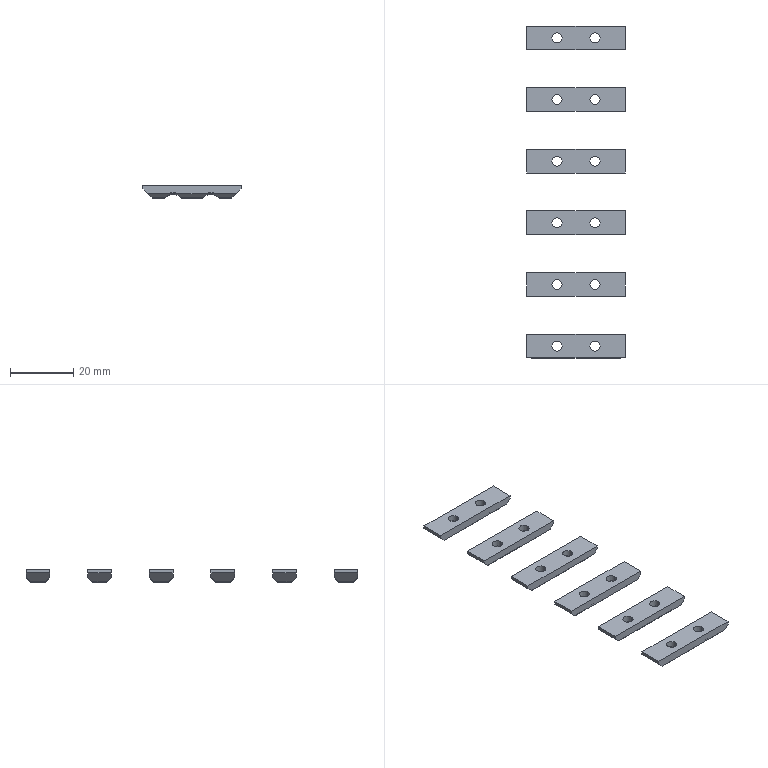NC program | NX | posted with a generic post | part box 31 x 105 x 4 mm
Lines 1 to 1424 of 12738:
N10 G17 G21 G94 G90
(FLOOR_WALL_COPY , TOOL : D10JING)
N12 T14 M6
N14 G54
N16 G17 G0 G90 X-65.5 Y18.497 S9500 M3
N18 G43 Z30. H14
N20 Z4.
N22 G94 G1 Z1. F1500.
N24 X-60.5
N26 X60.5
N28 Y11.898
N30 X-60.5
N32 Y5.298
N34 X60.5
N36 Y-1.301
N38 X-60.5
N40 Y-7.901
N42 X60.5
N44 Y-14.5
N46 X-60.5
N48 X-65.5
N50 Z4.
N52 G0 Z30.
N54 Y18.497
N56 Z3.
N58 G1 Z0.
N60 X-60.5
N62 X60.5
N64 Y11.898
N66 X-60.5
N68 Y5.298
N70 X60.5
N72 Y-1.301
N74 X-60.5
N76 Y-7.901
N78 X60.5
N80 Y-14.5
N82 X-60.5
N84 X-65.5
N86 Z3.
N88 G0 Z30.
N90 M5
(ZLEVEL_PROFILE_1 , TOOL : D10)
N92 T15 M6
N94 G54
N96 G17 G0 G90 X39.9 Y9.729 S9500 M3
N98 G43 Z30. H15
N100 Z1.5
N102 G94 G1 Y16.054 Z1.169 F1000.
N104 X40.234 Y17.398 Z1.096
N106 X40.916 Y18.604 Z1.023
N108 X41.896 Y19.584 Z0.951
N110 X43.102 Y20.266 Z0.878
N112 X44.446 Y20.6 Z0.805
N114 X53.054 Z0.354
N116 X54.398 Y20.266 Z0.282
N118 X55.604 Y19.584 Z0.209
N120 X56.584 Y18.604 Z0.137
N122 X57.266 Y17.398 Z0.064
N124 X57.6 Y16.054 Z-0.009
N126 Y0. Z-0.85
N128 Y-15.5 F2500.
N130 G2 X52.5 Y-20.6 R5.1
N132 G1 X45.
N134 G2 X39.9 Y-15.5 R5.1
N136 G1 Y15.5
N138 G2 X45. Y20.6 R5.1
N140 G1 X52.5
N142 G2 X57.6 Y15.5 R5.1
N144 G1 Y0.
N146 Y-15.459 Z-1.12
N148 X57.588 Y-15.845 Z-1.127
N150 X57.548 Y-16.23 Z-1.133
N152 X57.478 Y-16.61 Z-1.14
N154 X57.38 Y-16.983 Z-1.147
N156 X57.253 Y-17.349 Z-1.154
N158 X57.1 Y-17.703 Z-1.16
N160 X56.92 Y-18.045 Z-1.167
N162 X56.714 Y-18.372 Z-1.174
N164 X56.485 Y-18.683 Z-1.181
N166 X56.232 Y-18.976 Z-1.187
N168 X55.958 Y-19.248 Z-1.194
N170 X55.665 Y-19.499 Z-1.201
N172 X55.353 Y-19.727 Z-1.208
N174 X55.025 Y-19.931 Z-1.214
N176 X54.682 Y-20.11 Z-1.221
N178 X54.327 Y-20.262 Z-1.228
N180 X53.961 Y-20.386 Z-1.235
N182 X53.587 Y-20.483 Z-1.241
N184 X53.206 Y-20.551 Z-1.248
N186 X52.822 Y-20.59 Z-1.255
N188 X52.436 Y-20.6 Z-1.262
N190 X52.049 Z-1.268
N192 X45.093 Z-1.39
N194 X44.706 Y-20.592 Z-1.396
N196 X44.322 Y-20.555 Z-1.403
N198 X43.941 Y-20.489 Z-1.41
N200 X43.566 Y-20.394 Z-1.417
N202 X43.2 Y-20.272 Z-1.423
N204 X42.844 Y-20.122 Z-1.43
N206 X42.5 Y-19.945 Z-1.437
N208 X42.171 Y-19.743 Z-1.444
N210 X41.858 Y-19.517 Z-1.45
N212 X41.563 Y-19.267 Z-1.457
N214 X41.287 Y-18.996 Z-1.464
N216 X41.033 Y-18.705 Z-1.471
N218 X40.802 Y-18.396 Z-1.477
N220 X40.595 Y-18.07 Z-1.484
N222 X40.413 Y-17.729 Z-1.491
N224 X40.257 Y-17.375 Z-1.498
N226 X40.129 Y-17.011 Z-1.504
N228 X40.028 Y-16.637 Z-1.511
N230 X39.957 Y-16.258 Z-1.518
N232 X39.914 Y-15.874 Z-1.525
N234 X39.9 Y-15.488 Z-1.531
N236 Y-15.101 Z-1.538
N238 Y-5.826 Z-1.7
N240 Y15.5
N242 G2 X45. Y20.6 R5.1
N244 G1 X52.5
N246 G2 X57.6 Y15.5 R5.1
N248 G1 Y0.
N250 Y-15.459 Z-1.97
N252 X57.588 Y-15.845 Z-1.977
N254 X57.548 Y-16.23 Z-1.983
N256 X57.478 Y-16.61 Z-1.99
N258 X57.38 Y-16.983 Z-1.997
N260 X57.253 Y-17.349 Z-2.004
N262 X57.1 Y-17.703 Z-2.01
N264 X56.92 Y-18.045 Z-2.017
N266 X56.714 Y-18.372 Z-2.024
N268 X56.485 Y-18.683 Z-2.031
N270 X56.232 Y-18.976 Z-2.037
N272 X55.958 Y-19.248 Z-2.044
N274 X55.665 Y-19.499 Z-2.051
N276 X55.353 Y-19.727 Z-2.058
N278 X55.025 Y-19.931 Z-2.064
N280 X54.682 Y-20.11 Z-2.071
N282 X54.327 Y-20.262 Z-2.078
N284 X53.961 Y-20.386 Z-2.085
N286 X53.587 Y-20.483 Z-2.091
N288 X53.206 Y-20.551 Z-2.098
N290 X52.822 Y-20.59 Z-2.105
N292 X52.436 Y-20.6 Z-2.112
N294 X52.049 Z-2.118
N296 X45.093 Z-2.24
N298 X44.706 Y-20.592 Z-2.246
N300 X44.322 Y-20.555 Z-2.253
N302 X43.941 Y-20.489 Z-2.26
N304 X43.566 Y-20.394 Z-2.267
N306 X43.2 Y-20.272 Z-2.273
N308 X42.844 Y-20.122 Z-2.28
N310 X42.5 Y-19.945 Z-2.287
N312 X42.171 Y-19.743 Z-2.294
N314 X41.858 Y-19.517 Z-2.3
N316 X41.563 Y-19.267 Z-2.307
N318 X41.287 Y-18.996 Z-2.314
N320 X41.033 Y-18.705 Z-2.321
N322 X40.802 Y-18.396 Z-2.327
N324 X40.595 Y-18.07 Z-2.334
N326 X40.413 Y-17.729 Z-2.341
N328 X40.257 Y-17.375 Z-2.348
N330 X40.129 Y-17.011 Z-2.354
N332 X40.028 Y-16.637 Z-2.361
N334 X39.957 Y-16.258 Z-2.368
N336 X39.914 Y-15.874 Z-2.375
N338 X39.9 Y-15.488 Z-2.381
N340 Y-15.101 Z-2.388
N342 Y-5.826 Z-2.55
N344 Y15.5
N346 G2 X45. Y20.6 R5.1
N348 G1 X52.5
N350 G2 X57.6 Y15.5 R5.1
N352 G1 Y0.
N354 Y-15.459 Z-2.82
N356 X57.588 Y-15.845 Z-2.827
N358 X57.548 Y-16.23 Z-2.833
N360 X57.478 Y-16.61 Z-2.84
N362 X57.38 Y-16.983 Z-2.847
N364 X57.253 Y-17.349 Z-2.854
N366 X57.1 Y-17.703 Z-2.86
N368 X56.92 Y-18.045 Z-2.867
N370 X56.714 Y-18.372 Z-2.874
N372 X56.485 Y-18.683 Z-2.881
N374 X56.232 Y-18.976 Z-2.887
N376 X55.958 Y-19.248 Z-2.894
N378 X55.665 Y-19.499 Z-2.901
N380 X55.353 Y-19.727 Z-2.908
N382 X55.025 Y-19.931 Z-2.914
N384 X54.682 Y-20.11 Z-2.921
N386 X54.327 Y-20.262 Z-2.928
N388 X53.961 Y-20.386 Z-2.935
N390 X53.587 Y-20.483 Z-2.941
N392 X53.206 Y-20.551 Z-2.948
N394 X52.822 Y-20.59 Z-2.955
N396 X52.436 Y-20.6 Z-2.962
N398 X52.049 Z-2.968
N400 X45.093 Z-3.09
N402 X44.706 Y-20.592 Z-3.096
N404 X44.322 Y-20.555 Z-3.103
N406 X43.941 Y-20.489 Z-3.11
N408 X43.566 Y-20.394 Z-3.117
N410 X43.2 Y-20.272 Z-3.123
N412 X42.844 Y-20.122 Z-3.13
N414 X42.5 Y-19.945 Z-3.137
N416 X42.171 Y-19.743 Z-3.144
N418 X41.858 Y-19.517 Z-3.15
N420 X41.563 Y-19.267 Z-3.157
N422 X41.287 Y-18.996 Z-3.164
N424 X41.033 Y-18.705 Z-3.171
N426 X40.802 Y-18.396 Z-3.177
N428 X40.595 Y-18.07 Z-3.184
N430 X40.413 Y-17.729 Z-3.191
N432 X40.257 Y-17.375 Z-3.198
N434 X40.129 Y-17.011 Z-3.204
N436 X40.028 Y-16.637 Z-3.211
N438 X39.957 Y-16.258 Z-3.218
N440 X39.914 Y-15.874 Z-3.225
N442 X39.9 Y-15.488 Z-3.231
N444 Y-15.101 Z-3.238
N446 Y-5.826 Z-3.4
N448 Y15.5
N450 G2 X45. Y20.6 R5.1
N452 G1 X52.5
N454 G2 X57.6 Y15.5 R5.1
N456 G1 Y-15.5
N458 G2 X52.5 Y-20.6 R5.1
N460 G1 X45.
N462 G2 X39.9 Y-15.5 R5.1
N464 G1 Y-5.826
N466 Z-1.9
N468 G0 Z30.
N470 X-39.9 Y-9.729
N472 Z1.5
N474 G1 Y-16.054 Z1.169 F1000.
N476 X-40.234 Y-17.398 Z1.096
N478 X-40.916 Y-18.604 Z1.023
N480 X-41.896 Y-19.584 Z0.951
N482 X-43.102 Y-20.266 Z0.878
N484 X-44.446 Y-20.6 Z0.805
N486 X-53.054 Z0.354
N488 X-54.398 Y-20.266 Z0.282
N490 X-55.604 Y-19.584 Z0.209
N492 X-56.584 Y-18.604 Z0.137
N494 X-57.266 Y-17.398 Z0.064
N496 X-57.6 Y-16.054 Z-0.009
N498 Y0. Z-0.85
N500 Y15.5 F2500.
N502 G2 X-52.5 Y20.6 R5.1
N504 G1 X-45.
N506 G2 X-39.9 Y15.5 R5.1
N508 G1 Y-15.5
N510 G2 X-45. Y-20.6 R5.1
N512 G1 X-52.5
N514 G2 X-57.6 Y-15.5 R5.1
N516 G1 Y0.
N518 Y15.459 Z-1.12
N520 X-57.588 Y15.845 Z-1.127
N522 X-57.548 Y16.23 Z-1.133
N524 X-57.478 Y16.61 Z-1.14
N526 X-57.38 Y16.983 Z-1.147
N528 X-57.253 Y17.349 Z-1.154
N530 X-57.1 Y17.703 Z-1.16
N532 X-56.92 Y18.045 Z-1.167
N534 X-56.714 Y18.372 Z-1.174
N536 X-56.485 Y18.683 Z-1.181
N538 X-56.232 Y18.976 Z-1.187
N540 X-55.958 Y19.248 Z-1.194
N542 X-55.665 Y19.499 Z-1.201
N544 X-55.353 Y19.727 Z-1.208
N546 X-55.025 Y19.931 Z-1.214
N548 X-54.682 Y20.11 Z-1.221
N550 X-54.327 Y20.262 Z-1.228
N552 X-53.961 Y20.386 Z-1.235
N554 X-53.587 Y20.483 Z-1.241
N556 X-53.206 Y20.551 Z-1.248
N558 X-52.822 Y20.59 Z-1.255
N560 X-52.436 Y20.6 Z-1.262
N562 X-52.049 Z-1.268
N564 X-45.093 Z-1.39
N566 X-44.706 Y20.592 Z-1.396
N568 X-44.322 Y20.555 Z-1.403
N570 X-43.941 Y20.489 Z-1.41
N572 X-43.566 Y20.394 Z-1.417
N574 X-43.2 Y20.272 Z-1.423
N576 X-42.844 Y20.122 Z-1.43
N578 X-42.5 Y19.945 Z-1.437
N580 X-42.171 Y19.743 Z-1.444
N582 X-41.858 Y19.517 Z-1.45
N584 X-41.563 Y19.267 Z-1.457
N586 X-41.287 Y18.996 Z-1.464
N588 X-41.033 Y18.705 Z-1.471
N590 X-40.802 Y18.396 Z-1.477
N592 X-40.595 Y18.07 Z-1.484
N594 X-40.413 Y17.729 Z-1.491
N596 X-40.257 Y17.375 Z-1.498
N598 X-40.129 Y17.011 Z-1.504
N600 X-40.028 Y16.637 Z-1.511
N602 X-39.957 Y16.258 Z-1.518
N604 X-39.914 Y15.874 Z-1.525
N606 X-39.9 Y15.488 Z-1.531
N608 Y15.101 Z-1.538
N610 Y5.826 Z-1.7
N612 Y-15.5
N614 G2 X-45. Y-20.6 R5.1
N616 G1 X-52.5
N618 G2 X-57.6 Y-15.5 R5.1
N620 G1 Y0.
N622 Y15.459 Z-1.97
N624 X-57.588 Y15.845 Z-1.977
N626 X-57.548 Y16.23 Z-1.983
N628 X-57.478 Y16.61 Z-1.99
N630 X-57.38 Y16.983 Z-1.997
N632 X-57.253 Y17.349 Z-2.004
N634 X-57.1 Y17.703 Z-2.01
N636 X-56.92 Y18.045 Z-2.017
N638 X-56.714 Y18.372 Z-2.024
N640 X-56.485 Y18.683 Z-2.031
N642 X-56.232 Y18.976 Z-2.037
N644 X-55.958 Y19.248 Z-2.044
N646 X-55.665 Y19.499 Z-2.051
N648 X-55.353 Y19.727 Z-2.058
N650 X-55.025 Y19.931 Z-2.064
N652 X-54.682 Y20.11 Z-2.071
N654 X-54.327 Y20.262 Z-2.078
N656 X-53.961 Y20.386 Z-2.085
N658 X-53.587 Y20.483 Z-2.091
N660 X-53.206 Y20.551 Z-2.098
N662 X-52.822 Y20.59 Z-2.105
N664 X-52.436 Y20.6 Z-2.112
N666 X-52.049 Z-2.118
N668 X-45.093 Z-2.24
N670 X-44.706 Y20.592 Z-2.246
N672 X-44.322 Y20.555 Z-2.253
N674 X-43.941 Y20.489 Z-2.26
N676 X-43.566 Y20.394 Z-2.267
N678 X-43.2 Y20.272 Z-2.273
N680 X-42.844 Y20.122 Z-2.28
N682 X-42.5 Y19.945 Z-2.287
N684 X-42.171 Y19.743 Z-2.294
N686 X-41.858 Y19.517 Z-2.3
N688 X-41.563 Y19.267 Z-2.307
N690 X-41.287 Y18.996 Z-2.314
N692 X-41.033 Y18.705 Z-2.321
N694 X-40.802 Y18.396 Z-2.327
N696 X-40.595 Y18.07 Z-2.334
N698 X-40.413 Y17.729 Z-2.341
N700 X-40.257 Y17.375 Z-2.348
N702 X-40.129 Y17.011 Z-2.354
N704 X-40.028 Y16.637 Z-2.361
N706 X-39.957 Y16.258 Z-2.368
N708 X-39.914 Y15.874 Z-2.375
N710 X-39.9 Y15.488 Z-2.381
N712 Y15.101 Z-2.388
N714 Y5.826 Z-2.55
N716 Y-15.5
N718 G2 X-45. Y-20.6 R5.1
N720 G1 X-52.5
N722 G2 X-57.6 Y-15.5 R5.1
N724 G1 Y0.
N726 Y15.459 Z-2.82
N728 X-57.588 Y15.845 Z-2.827
N730 X-57.548 Y16.23 Z-2.833
N732 X-57.478 Y16.61 Z-2.84
N734 X-57.38 Y16.983 Z-2.847
N736 X-57.253 Y17.349 Z-2.854
N738 X-57.1 Y17.703 Z-2.86
N740 X-56.92 Y18.045 Z-2.867
N742 X-56.714 Y18.372 Z-2.874
N744 X-56.485 Y18.683 Z-2.881
N746 X-56.232 Y18.976 Z-2.887
N748 X-55.958 Y19.248 Z-2.894
N750 X-55.665 Y19.499 Z-2.901
N752 X-55.353 Y19.727 Z-2.908
N754 X-55.025 Y19.931 Z-2.914
N756 X-54.682 Y20.11 Z-2.921
N758 X-54.327 Y20.262 Z-2.928
N760 X-53.961 Y20.386 Z-2.935
N762 X-53.587 Y20.483 Z-2.941
N764 X-53.206 Y20.551 Z-2.948
N766 X-52.822 Y20.59 Z-2.955
N768 X-52.436 Y20.6 Z-2.962
N770 X-52.049 Z-2.968
N772 X-45.093 Z-3.09
N774 X-44.706 Y20.592 Z-3.096
N776 X-44.322 Y20.555 Z-3.103
N778 X-43.941 Y20.489 Z-3.11
N780 X-43.566 Y20.394 Z-3.117
N782 X-43.2 Y20.272 Z-3.123
N784 X-42.844 Y20.122 Z-3.13
N786 X-42.5 Y19.945 Z-3.137
N788 X-42.171 Y19.743 Z-3.144
N790 X-41.858 Y19.517 Z-3.15
N792 X-41.563 Y19.267 Z-3.157
N794 X-41.287 Y18.996 Z-3.164
N796 X-41.033 Y18.705 Z-3.171
N798 X-40.802 Y18.396 Z-3.177
N800 X-40.595 Y18.07 Z-3.184
N802 X-40.413 Y17.729 Z-3.191
N804 X-40.257 Y17.375 Z-3.198
N806 X-40.129 Y17.011 Z-3.204
N808 X-40.028 Y16.637 Z-3.211
N810 X-39.957 Y16.258 Z-3.218
N812 X-39.914 Y15.874 Z-3.225
N814 X-39.9 Y15.488 Z-3.231
N816 Y15.101 Z-3.238
N818 Y5.826 Z-3.4
N820 Y-15.5
N822 G2 X-45. Y-20.6 R5.1
N824 G1 X-52.5
N826 G2 X-57.6 Y-15.5 R5.1
N828 G1 Y15.5
N830 G2 X-52.5 Y20.6 R5.1
N832 G1 X-45.
N834 G2 X-39.9 Y15.5 R5.1
N836 G1 Y5.826
N838 Z-1.9
N840 G0 Z30.
N842 X-20.4 Y-9.729
N844 Z1.5
N846 G1 Y-16.054 Z1.169 F1000.
N848 X-20.734 Y-17.398 Z1.096
N850 X-21.416 Y-18.604 Z1.023
N852 X-22.396 Y-19.584 Z0.951
N854 X-23.602 Y-20.266 Z0.878
N856 X-24.946 Y-20.6 Z0.805
N858 X-33.554 Z0.354
N860 X-34.898 Y-20.266 Z0.282
N862 X-36.104 Y-19.584 Z0.209
N864 X-37.084 Y-18.604 Z0.137
N866 X-37.766 Y-17.398 Z0.064
N868 X-38.1 Y-16.054 Z-0.009
N870 Y0. Z-0.85
N872 Y15.5 F2500.
N874 G2 X-33. Y20.6 R5.1
N876 G1 X-25.5
N878 G2 X-20.4 Y15.5 R5.1
N880 G1 Y-15.5
N882 G2 X-25.5 Y-20.6 R5.1
N884 G1 X-33.
N886 G2 X-38.1 Y-15.5 R5.1
N888 G1 Y0.
N890 Y15.459 Z-1.12
N892 X-38.088 Y15.845 Z-1.127
N894 X-38.048 Y16.23 Z-1.133
N896 X-37.978 Y16.61 Z-1.14
N898 X-37.88 Y16.983 Z-1.147
N900 X-37.753 Y17.349 Z-1.154
N902 X-37.6 Y17.703 Z-1.16
N904 X-37.42 Y18.045 Z-1.167
N906 X-37.214 Y18.372 Z-1.174
N908 X-36.985 Y18.683 Z-1.181
N910 X-36.732 Y18.976 Z-1.187
N912 X-36.458 Y19.248 Z-1.194
N914 X-36.165 Y19.499 Z-1.201
N916 X-35.853 Y19.727 Z-1.208
N918 X-35.525 Y19.931 Z-1.214
N920 X-35.182 Y20.11 Z-1.221
N922 X-34.827 Y20.262 Z-1.228
N924 X-34.461 Y20.386 Z-1.235
N926 X-34.087 Y20.483 Z-1.241
N928 X-33.706 Y20.551 Z-1.248
N930 X-33.322 Y20.59 Z-1.255
N932 X-32.936 Y20.6 Z-1.262
N934 X-32.549 Z-1.268
N936 X-25.593 Z-1.39
N938 X-25.206 Y20.592 Z-1.396
N940 X-24.822 Y20.555 Z-1.403
N942 X-24.441 Y20.489 Z-1.41
N944 X-24.066 Y20.394 Z-1.417
N946 X-23.7 Y20.272 Z-1.423
N948 X-23.344 Y20.122 Z-1.43
N950 X-23. Y19.945 Z-1.437
N952 X-22.671 Y19.743 Z-1.444
N954 X-22.358 Y19.517 Z-1.45
N956 X-22.063 Y19.267 Z-1.457
N958 X-21.787 Y18.996 Z-1.464
N960 X-21.533 Y18.705 Z-1.471
N962 X-21.302 Y18.396 Z-1.477
N964 X-21.095 Y18.07 Z-1.484
N966 X-20.913 Y17.729 Z-1.491
N968 X-20.757 Y17.375 Z-1.498
N970 X-20.629 Y17.011 Z-1.504
N972 X-20.528 Y16.637 Z-1.511
N974 X-20.457 Y16.258 Z-1.518
N976 X-20.414 Y15.874 Z-1.525
N978 X-20.4 Y15.488 Z-1.531
N980 Y15.101 Z-1.538
N982 Y5.826 Z-1.7
N984 Y-15.5
N986 G2 X-25.5 Y-20.6 R5.1
N988 G1 X-33.
N990 G2 X-38.1 Y-15.5 R5.1
N992 G1 Y0.
N994 Y15.459 Z-1.97
N996 X-38.088 Y15.845 Z-1.977
N998 X-38.048 Y16.23 Z-1.983
N1000 X-37.978 Y16.61 Z-1.99
N1002 X-37.88 Y16.983 Z-1.997
N1004 X-37.753 Y17.349 Z-2.004
N1006 X-37.6 Y17.703 Z-2.01
N1008 X-37.42 Y18.045 Z-2.017
N1010 X-37.214 Y18.372 Z-2.024
N1012 X-36.985 Y18.683 Z-2.031
N1014 X-36.732 Y18.976 Z-2.037
N1016 X-36.458 Y19.248 Z-2.044
N1018 X-36.165 Y19.499 Z-2.051
N1020 X-35.853 Y19.727 Z-2.058
N1022 X-35.525 Y19.931 Z-2.064
N1024 X-35.182 Y20.11 Z-2.071
N1026 X-34.827 Y20.262 Z-2.078
N1028 X-34.461 Y20.386 Z-2.085
N1030 X-34.087 Y20.483 Z-2.091
N1032 X-33.706 Y20.551 Z-2.098
N1034 X-33.322 Y20.59 Z-2.105
N1036 X-32.936 Y20.6 Z-2.112
N1038 X-32.549 Z-2.118
N1040 X-25.593 Z-2.24
N1042 X-25.206 Y20.592 Z-2.246
N1044 X-24.822 Y20.555 Z-2.253
N1046 X-24.441 Y20.489 Z-2.26
N1048 X-24.066 Y20.394 Z-2.267
N1050 X-23.7 Y20.272 Z-2.273
N1052 X-23.344 Y20.122 Z-2.28
N1054 X-23. Y19.945 Z-2.287
N1056 X-22.671 Y19.743 Z-2.294
N1058 X-22.358 Y19.517 Z-2.3
N1060 X-22.063 Y19.267 Z-2.307
N1062 X-21.787 Y18.996 Z-2.314
N1064 X-21.533 Y18.705 Z-2.321
N1066 X-21.302 Y18.396 Z-2.327
N1068 X-21.095 Y18.07 Z-2.334
N1070 X-20.913 Y17.729 Z-2.341
N1072 X-20.757 Y17.375 Z-2.348
N1074 X-20.629 Y17.011 Z-2.354
N1076 X-20.528 Y16.637 Z-2.361
N1078 X-20.457 Y16.258 Z-2.368
N1080 X-20.414 Y15.874 Z-2.375
N1082 X-20.4 Y15.488 Z-2.381
N1084 Y15.101 Z-2.388
N1086 Y5.826 Z-2.55
N1088 Y-15.5
N1090 G2 X-25.5 Y-20.6 R5.1
N1092 G1 X-33.
N1094 G2 X-38.1 Y-15.5 R5.1
N1096 G1 Y0.
N1098 Y15.459 Z-2.82
N1100 X-38.088 Y15.845 Z-2.827
N1102 X-38.048 Y16.23 Z-2.833
N1104 X-37.978 Y16.61 Z-2.84
N1106 X-37.88 Y16.983 Z-2.847
N1108 X-37.753 Y17.349 Z-2.854
N1110 X-37.6 Y17.703 Z-2.86
N1112 X-37.42 Y18.045 Z-2.867
N1114 X-37.214 Y18.372 Z-2.874
N1116 X-36.985 Y18.683 Z-2.881
N1118 X-36.732 Y18.976 Z-2.887
N1120 X-36.458 Y19.248 Z-2.894
N1122 X-36.165 Y19.499 Z-2.901
N1124 X-35.853 Y19.727 Z-2.908
N1126 X-35.525 Y19.931 Z-2.914
N1128 X-35.182 Y20.11 Z-2.921
N1130 X-34.827 Y20.262 Z-2.928
N1132 X-34.461 Y20.386 Z-2.935
N1134 X-34.087 Y20.483 Z-2.941
N1136 X-33.706 Y20.551 Z-2.948
N1138 X-33.322 Y20.59 Z-2.955
N1140 X-32.936 Y20.6 Z-2.962
N1142 X-32.549 Z-2.968
N1144 X-25.593 Z-3.09
N1146 X-25.206 Y20.592 Z-3.096
N1148 X-24.822 Y20.555 Z-3.103
N1150 X-24.441 Y20.489 Z-3.11
N1152 X-24.066 Y20.394 Z-3.117
N1154 X-23.7 Y20.272 Z-3.123
N1156 X-23.344 Y20.122 Z-3.13
N1158 X-23. Y19.945 Z-3.137
N1160 X-22.671 Y19.743 Z-3.144
N1162 X-22.358 Y19.517 Z-3.15
N1164 X-22.063 Y19.267 Z-3.157
N1166 X-21.787 Y18.996 Z-3.164
N1168 X-21.533 Y18.705 Z-3.171
N1170 X-21.302 Y18.396 Z-3.177
N1172 X-21.095 Y18.07 Z-3.184
N1174 X-20.913 Y17.729 Z-3.191
N1176 X-20.757 Y17.375 Z-3.198
N1178 X-20.629 Y17.011 Z-3.204
N1180 X-20.528 Y16.637 Z-3.211
N1182 X-20.457 Y16.258 Z-3.218
N1184 X-20.414 Y15.874 Z-3.225
N1186 X-20.4 Y15.488 Z-3.231
N1188 Y15.101 Z-3.238
N1190 Y5.826 Z-3.4
N1192 Y-15.5
N1194 G2 X-25.5 Y-20.6 R5.1
N1196 G1 X-33.
N1198 G2 X-38.1 Y-15.5 R5.1
N1200 G1 Y15.5
N1202 G2 X-33. Y20.6 R5.1
N1204 G1 X-25.5
N1206 G2 X-20.4 Y15.5 R5.1
N1208 G1 Y5.826
N1210 Z-1.9
N1212 G0 Z30.
N1214 X-0.9 Y-9.729
N1216 Z1.5
N1218 G1 Y-16.054 Z1.169 F1000.
N1220 X-1.234 Y-17.398 Z1.096
N1222 X-1.916 Y-18.604 Z1.023
N1224 X-2.896 Y-19.584 Z0.951
N1226 X-4.102 Y-20.266 Z0.878
N1228 X-5.446 Y-20.6 Z0.805
N1230 X-14.054 Z0.354
N1232 X-15.398 Y-20.266 Z0.282
N1234 X-16.604 Y-19.584 Z0.209
N1236 X-17.584 Y-18.604 Z0.137
N1238 X-18.266 Y-17.398 Z0.064
N1240 X-18.6 Y-16.054 Z-0.009
N1242 Y0. Z-0.85
N1244 Y15.5 F2500.
N1246 G2 X-13.5 Y20.6 R5.1
N1248 G1 X-6.
N1250 G2 X-0.9 Y15.5 R5.1
N1252 G1 Y-15.5
N1254 G2 X-6. Y-20.6 R5.1
N1256 G1 X-13.5
N1258 G2 X-18.6 Y-15.5 R5.1
N1260 G1 Y0.
N1262 Y15.459 Z-1.12
N1264 X-18.588 Y15.845 Z-1.127
N1266 X-18.548 Y16.23 Z-1.133
N1268 X-18.478 Y16.61 Z-1.14
N1270 X-18.38 Y16.983 Z-1.147
N1272 X-18.253 Y17.349 Z-1.154
N1274 X-18.1 Y17.703 Z-1.16
N1276 X-17.92 Y18.045 Z-1.167
N1278 X-17.714 Y18.372 Z-1.174
N1280 X-17.485 Y18.683 Z-1.181
N1282 X-17.232 Y18.976 Z-1.187
N1284 X-16.958 Y19.248 Z-1.194
N1286 X-16.665 Y19.499 Z-1.201
N1288 X-16.353 Y19.727 Z-1.208
N1290 X-16.025 Y19.931 Z-1.214
N1292 X-15.682 Y20.11 Z-1.221
N1294 X-15.327 Y20.262 Z-1.228
N1296 X-14.961 Y20.386 Z-1.235
N1298 X-14.587 Y20.483 Z-1.241
N1300 X-14.206 Y20.551 Z-1.248
N1302 X-13.822 Y20.59 Z-1.255
N1304 X-13.436 Y20.6 Z-1.262
N1306 X-13.049 Z-1.268
N1308 X-6.093 Z-1.39
N1310 X-5.706 Y20.592 Z-1.396
N1312 X-5.322 Y20.555 Z-1.403
N1314 X-4.941 Y20.489 Z-1.41
N1316 X-4.566 Y20.394 Z-1.417
N1318 X-4.2 Y20.272 Z-1.423
N1320 X-3.844 Y20.122 Z-1.43
N1322 X-3.5 Y19.945 Z-1.437
N1324 X-3.171 Y19.743 Z-1.444
N1326 X-2.858 Y19.517 Z-1.45
N1328 X-2.563 Y19.267 Z-1.457
N1330 X-2.287 Y18.996 Z-1.464
N1332 X-2.033 Y18.705 Z-1.471
N1334 X-1.802 Y18.396 Z-1.477
N1336 X-1.595 Y18.07 Z-1.484
N1338 X-1.413 Y17.729 Z-1.491
N1340 X-1.257 Y17.375 Z-1.498
N1342 X-1.129 Y17.011 Z-1.504
N1344 X-1.028 Y16.637 Z-1.511
N1346 X-0.957 Y16.258 Z-1.518
N1348 X-0.914 Y15.874 Z-1.525
N1350 X-0.9 Y15.488 Z-1.531
N1352 Y15.101 Z-1.538
N1354 Y5.826 Z-1.7
N1356 Y-15.5
N1358 G2 X-6. Y-20.6 R5.1
N1360 G1 X-13.5
N1362 G2 X-18.6 Y-15.5 R5.1
N1364 G1 Y0.
N1366 Y15.459 Z-1.97
N1368 X-18.588 Y15.845 Z-1.977
N1370 X-18.548 Y16.23 Z-1.983
N1372 X-18.478 Y16.61 Z-1.99
N1374 X-18.38 Y16.983 Z-1.997
N1376 X-18.253 Y17.349 Z-2.004
N1378 X-18.1 Y17.703 Z-2.01
N1380 X-17.92 Y18.045 Z-2.017
N1382 X-17.714 Y18.372 Z-2.024
N1384 X-17.485 Y18.683 Z-2.031
N1386 X-17.232 Y18.976 Z-2.037
N1388 X-16.958 Y19.248 Z-2.044
N1390 X-16.665 Y19.499 Z-2.051
N1392 X-16.353 Y19.727 Z-2.058
N1394 X-16.025 Y19.931 Z-2.064
N1396 X-15.682 Y20.11 Z-2.071
N1398 X-15.327 Y20.262 Z-2.078
N1400 X-14.961 Y20.386 Z-2.085
N1402 X-14.587 Y20.483 Z-2.091
N1404 X-14.206 Y20.551 Z-2.098
N1406 X-13.822 Y20.59 Z-2.105
N1408 X-13.436 Y20.6 Z-2.112
N1410 X-13.049 Z-2.118
N1412 X-6.093 Z-2.24
N1414 X-5.706 Y20.592 Z-2.246
N1416 X-5.322 Y20.555 Z-2.253
N1418 X-4.941 Y20.489 Z-2.26
N1420 X-4.566 Y20.394 Z-2.267
N1422 X-4.2 Y20.272 Z-2.273
N1424 X-3.844 Y20.122 Z-2.28
N1426 X-3.5 Y19.945 Z-2.287
N1428 X-3.171 Y19.743 Z-2.294
N1430 X-2.858 Y19.517 Z-2.3
N1432 X-2.563 Y19.267 Z-2.307
N1434 X-2.287 Y18.996 Z-2.314
N1436 X-2.033 Y18.705 Z-2.321
N1438 X-1.802 Y18.396 Z-2.327
N1440 X-1.595 Y18.07 Z-2.334
N1442 X-1.413 Y17.729 Z-2.341
N1444 X-1.257 Y17.375 Z-2.348
N1446 X-1.129 Y17.011 Z-2.354
N1448 X-1.028 Y16.637 Z-2.361
N1450 X-0.957 Y16.258 Z-2.368
N1452 X-0.914 Y15.874 Z-2.375
N1454 X-0.9 Y15.488 Z-2.381
N1456 Y15.101 Z-2.388
N1458 Y5.826 Z-2.55
N1460 Y-15.5
N1462 G2 X-6. Y-20.6 R5.1
N1464 G1 X-13.5
N1466 G2 X-18.6 Y-15.5 R5.1
N1468 G1 Y0.
N1470 Y15.459 Z-2.82
N1472 X-18.588 Y15.845 Z-2.827
N1474 X-18.548 Y16.23 Z-2.833
N1476 X-18.478 Y16.61 Z-2.84
N1478 X-18.38 Y16.983 Z-2.847
N1480 X-18.253 Y17.349 Z-2.854
N1482 X-18.1 Y17.703 Z-2.86
N1484 X-17.92 Y18.045 Z-2.867
N1486 X-17.714 Y18.372 Z-2.874
N1488 X-17.485 Y18.683 Z-2.881
N1490 X-17.232 Y18.976 Z-2.887
N1492 X-16.958 Y19.248 Z-2.894
N1494 X-16.665 Y19.499 Z-2.901
N1496 X-16.353 Y19.727 Z-2.908
N1498 X-16.025 Y19.931 Z-2.914
N1500 X-15.682 Y20.11 Z-2.921
N1502 X-15.327 Y20.262 Z-2.928
N1504 X-14.961 Y20.386 Z-2.935
N1506 X-14.587 Y20.483 Z-2.941
N1508 X-14.206 Y20.551 Z-2.948
N1510 X-13.822 Y20.59 Z-2.955
N1512 X-13.436 Y20.6 Z-2.962
N1514 X-13.049 Z-2.968
N1516 X-6.093 Z-3.09
N1518 X-5.706 Y20.592 Z-3.096
N1520 X-5.322 Y20.555 Z-3.103
N1522 X-4.941 Y20.489 Z-3.11
N1524 X-4.566 Y20.394 Z-3.117
N1526 X-4.2 Y20.272 Z-3.123
N1528 X-3.844 Y20.122 Z-3.13
N1530 X-3.5 Y19.945 Z-3.137
N1532 X-3.171 Y19.743 Z-3.144
N1534 X-2.858 Y19.517 Z-3.15
N1536 X-2.563 Y19.267 Z-3.157
N1538 X-2.287 Y18.996 Z-3.164
N1540 X-2.033 Y18.705 Z-3.171
N1542 X-1.802 Y18.396 Z-3.177
N1544 X-1.595 Y18.07 Z-3.184
N1546 X-1.413 Y17.729 Z-3.191
N1548 X-1.257 Y17.375 Z-3.198
N1550 X-1.129 Y17.011 Z-3.204
N1552 X-1.028 Y16.637 Z-3.211
N1554 X-0.957 Y16.258 Z-3.218
N1556 X-0.914 Y15.874 Z-3.225
N1558 X-0.9 Y15.488 Z-3.231
N1560 Y15.101 Z-3.238
N1562 Y5.826 Z-3.4
N1564 Y-15.5
N1566 G2 X-6. Y-20.6 R5.1
N1568 G1 X-13.5
N1570 G2 X-18.6 Y-15.5 R5.1
N1572 G1 Y15.5
N1574 G2 X-13.5 Y20.6 R5.1
N1576 G1 X-6.
N1578 G2 X-0.9 Y15.5 R5.1
N1580 G1 Y5.826
N1582 Z-1.9
N1584 G0 Z30.
N1586 X18.6 Y-9.729
N1588 Z1.5
N1590 G1 Y-16.054 Z1.169 F1000.
N1592 X18.266 Y-17.398 Z1.096
N1594 X17.584 Y-18.604 Z1.023
N1596 X16.604 Y-19.584 Z0.951
N1598 X15.398 Y-20.266 Z0.878
N1600 X14.054 Y-20.6 Z0.805
N1602 X5.446 Z0.354
N1604 X4.102 Y-20.266 Z0.282
N1606 X2.896 Y-19.584 Z0.209
N1608 X1.916 Y-18.604 Z0.137
N1610 X1.234 Y-17.398 Z0.064
N1612 X0.9 Y-16.054 Z-0.009
N1614 Y0. Z-0.85
N1616 Y15.5 F2500.
N1618 G2 X6. Y20.6 R5.1
N1620 G1 X13.5
N1622 G2 X18.6 Y15.5 R5.1
N1624 G1 Y-15.5
N1626 G2 X13.5 Y-20.6 R5.1
N1628 G1 X6.
N1630 G2 X0.9 Y-15.5 R5.1
N1632 G1 Y0.
N1634 Y15.459 Z-1.12
N1636 X0.912 Y15.845 Z-1.127
N1638 X0.952 Y16.23 Z-1.133
N1640 X1.022 Y16.61 Z-1.14
N1642 X1.12 Y16.983 Z-1.147
N1644 X1.247 Y17.349 Z-1.154
N1646 X1.4 Y17.703 Z-1.16
N1648 X1.58 Y18.045 Z-1.167
N1650 X1.786 Y18.372 Z-1.174
N1652 X2.015 Y18.683 Z-1.181
N1654 X2.268 Y18.976 Z-1.187
N1656 X2.542 Y19.248 Z-1.194
N1658 X2.835 Y19.499 Z-1.201
N1660 X3.147 Y19.727 Z-1.208
N1662 X3.475 Y19.931 Z-1.214
N1664 X3.818 Y20.11 Z-1.221
N1666 X4.173 Y20.262 Z-1.228
N1668 X4.539 Y20.386 Z-1.235
N1670 X4.913 Y20.483 Z-1.241
N1672 X5.294 Y20.551 Z-1.248
N1674 X5.678 Y20.59 Z-1.255
N1676 X6.064 Y20.6 Z-1.262
N1678 X6.451 Z-1.268
N1680 X13.407 Z-1.39
N1682 X13.794 Y20.592 Z-1.396
N1684 X14.178 Y20.555 Z-1.403
N1686 X14.559 Y20.489 Z-1.41
N1688 X14.934 Y20.394 Z-1.417
N1690 X15.3 Y20.272 Z-1.423
N1692 X15.656 Y20.122 Z-1.43
N1694 X16. Y19.945 Z-1.437
N1696 X16.329 Y19.743 Z-1.444
N1698 X16.642 Y19.517 Z-1.45
N1700 X16.937 Y19.267 Z-1.457
N1702 X17.213 Y18.996 Z-1.464
N1704 X17.467 Y18.705 Z-1.471
N1706 X17.698 Y18.396 Z-1.477
N1708 X17.905 Y18.07 Z-1.484
N1710 X18.087 Y17.729 Z-1.491
N1712 X18.243 Y17.375 Z-1.498
N1714 X18.371 Y17.011 Z-1.504
N1716 X18.472 Y16.637 Z-1.511
N1718 X18.543 Y16.258 Z-1.518
N1720 X18.586 Y15.874 Z-1.525
N1722 X18.6 Y15.488 Z-1.531
N1724 Y15.101 Z-1.538
N1726 Y5.826 Z-1.7
N1728 Y-15.5
N1730 G2 X13.5 Y-20.6 R5.1
N1732 G1 X6.
N1734 G2 X0.9 Y-15.5 R5.1
N1736 G1 Y0.
N1738 Y15.459 Z-1.97
N1740 X0.912 Y15.845 Z-1.977
N1742 X0.952 Y16.23 Z-1.983
N1744 X1.022 Y16.61 Z-1.99
N1746 X1.12 Y16.983 Z-1.997
N1748 X1.247 Y17.349 Z-2.004
N1750 X1.4 Y17.703 Z-2.01
N1752 X1.58 Y18.045 Z-2.017
N1754 X1.786 Y18.372 Z-2.024
N1756 X2.015 Y18.683 Z-2.031
N1758 X2.268 Y18.976 Z-2.037
N1760 X2.542 Y19.248 Z-2.044
N1762 X2.835 Y19.499 Z-2.051
N1764 X3.147 Y19.727 Z-2.058
N1766 X3.475 Y19.931 Z-2.064
N1768 X3.818 Y20.11 Z-2.071
N1770 X4.173 Y20.262 Z-2.078
N1772 X4.539 Y20.386 Z-2.085
N1774 X4.913 Y20.483 Z-2.091
N1776 X5.294 Y20.551 Z-2.098
N1778 X5.678 Y20.59 Z-2.105
N1780 X6.064 Y20.6 Z-2.112
N1782 X6.451 Z-2.118
N1784 X13.407 Z-2.24
N1786 X13.794 Y20.592 Z-2.246
N1788 X14.178 Y20.555 Z-2.253
N1790 X14.559 Y20.489 Z-2.26
N1792 X14.934 Y20.394 Z-2.267
N1794 X15.3 Y20.272 Z-2.273
N1796 X15.656 Y20.122 Z-2.28
N1798 X16. Y19.945 Z-2.287
N1800 X16.329 Y19.743 Z-2.294
N1802 X16.642 Y19.517 Z-2.3
N1804 X16.937 Y19.267 Z-2.307
N1806 X17.213 Y18.996 Z-2.314
N1808 X17.467 Y18.705 Z-2.321
N1810 X17.698 Y18.396 Z-2.327
N1812 X17.905 Y18.07 Z-2.334
N1814 X18.087 Y17.729 Z-2.341
N1816 X18.243 Y17.375 Z-2.348
N1818 X18.371 Y17.011 Z-2.354
N1820 X18.472 Y16.637 Z-2.361
N1822 X18.543 Y16.258 Z-2.368
N1824 X18.586 Y15.874 Z-2.375
N1826 X18.6 Y15.488 Z-2.381
N1828 Y15.101 Z-2.388
N1830 Y5.826 Z-2.55
N1832 Y-15.5
N1834 G2 X13.5 Y-20.6 R5.1
N1836 G1 X6.
N1838 G2 X0.9 Y-15.5 R5.1
N1840 G1 Y0.
N1842 Y15.459 Z-2.82
N1844 X0.912 Y15.845 Z-2.827
N1846 X0.952 Y16.23 Z-2.833
N1848 X1.022 Y16.61 Z-2.84
N1850 X1.12 Y16.983 Z-2.847
N1852 X1.247 Y17.349 Z-2.854
N1854 X1.4 Y17.703 Z-2.86
N1856 X1.58 Y18.045 Z-2.867
N1858 X1.786 Y18.372 Z-2.874
N1860 X2.015 Y18.683 Z-2.881
N1862 X2.268 Y18.976 Z-2.887
N1864 X2.542 Y19.248 Z-2.894
N1866 X2.835 Y19.499 Z-2.901
N1868 X3.147 Y19.727 Z-2.908
N1870 X3.475 Y19.931 Z-2.914
N1872 X3.818 Y20.11 Z-2.921
N1874 X4.173 Y20.262 Z-2.928
N1876 X4.539 Y20.386 Z-2.935
N1878 X4.913 Y20.483 Z-2.941
N1880 X5.294 Y20.551 Z-2.948
N1882 X5.678 Y20.59 Z-2.955
N1884 X6.064 Y20.6 Z-2.962
N1886 X6.451 Z-2.968
N1888 X13.407 Z-3.09
N1890 X13.794 Y20.592 Z-3.096
N1892 X14.178 Y20.555 Z-3.103
N1894 X14.559 Y20.489 Z-3.11
N1896 X14.934 Y20.394 Z-3.117
N1898 X15.3 Y20.272 Z-3.123
N1900 X15.656 Y20.122 Z-3.13
N1902 X16. Y19.945 Z-3.137
N1904 X16.329 Y19.743 Z-3.144
N1906 X16.642 Y19.517 Z-3.15
N1908 X16.937 Y19.267 Z-3.157
N1910 X17.213 Y18.996 Z-3.164
N1912 X17.467 Y18.705 Z-3.171
N1914 X17.698 Y18.396 Z-3.177
N1916 X17.905 Y18.07 Z-3.184
N1918 X18.087 Y17.729 Z-3.191
N1920 X18.243 Y17.375 Z-3.198
N1922 X18.371 Y17.011 Z-3.204
N1924 X18.472 Y16.637 Z-3.211
N1926 X18.543 Y16.258 Z-3.218
N1928 X18.586 Y15.874 Z-3.225
N1930 X18.6 Y15.488 Z-3.231
N1932 Y15.101 Z-3.238
N1934 Y5.826 Z-3.4
N1936 Y-15.5
N1938 G2 X13.5 Y-20.6 R5.1
N1940 G1 X6.
N1942 G2 X0.9 Y-15.5 R5.1
N1944 G1 Y15.5
N1946 G2 X6. Y20.6 R5.1
N1948 G1 X13.5
N1950 G2 X18.6 Y15.5 R5.1
N1952 G1 Y5.826
N1954 Z-1.9
N1956 G0 Z30.
N1958 X38.1 Y-9.729
N1960 Z1.5
N1962 G1 Y-16.054 Z1.169 F1000.
N1964 X37.766 Y-17.398 Z1.096
N1966 X37.084 Y-18.604 Z1.023
N1968 X36.104 Y-19.584 Z0.951
N1970 X34.898 Y-20.266 Z0.878
N1972 X33.554 Y-20.6 Z0.805
N1974 X24.946 Z0.354
N1976 X23.602 Y-20.266 Z0.282
N1978 X22.396 Y-19.584 Z0.209
N1980 X21.416 Y-18.604 Z0.137
N1982 X20.734 Y-17.398 Z0.064
N1984 X20.4 Y-16.054 Z-0.009
N1986 Y0. Z-0.85
N1988 Y15.5 F2500.
N1990 G2 X25.5 Y20.6 R5.1
N1992 G1 X33.
N1994 G2 X38.1 Y15.5 R5.1
N1996 G1 Y-15.5
N1998 G2 X33. Y-20.6 R5.1
N2000 G1 X25.5
N2002 G2 X20.4 Y-15.5 R5.1
N2004 G1 Y0.
N2006 Y15.459 Z-1.12
N2008 X20.412 Y15.845 Z-1.127
N2010 X20.452 Y16.23 Z-1.133
N2012 X20.522 Y16.61 Z-1.14
N2014 X20.62 Y16.983 Z-1.147
N2016 X20.747 Y17.349 Z-1.154
N2018 X20.9 Y17.703 Z-1.16
N2020 X21.08 Y18.045 Z-1.167
N2022 X21.286 Y18.372 Z-1.174
N2024 X21.515 Y18.683 Z-1.181
N2026 X21.768 Y18.976 Z-1.187
N2028 X22.042 Y19.248 Z-1.194
N2030 X22.335 Y19.499 Z-1.201
N2032 X22.647 Y19.727 Z-1.208
N2034 X22.975 Y19.931 Z-1.214
N2036 X23.318 Y20.11 Z-1.221
N2038 X23.673 Y20.262 Z-1.228
N2040 X24.039 Y20.386 Z-1.235
N2042 X24.413 Y20.483 Z-1.241
N2044 X24.794 Y20.551 Z-1.248
N2046 X25.178 Y20.59 Z-1.255
N2048 X25.564 Y20.6 Z-1.262
N2050 X25.951 Z-1.268
N2052 X32.907 Z-1.39
N2054 X33.294 Y20.592 Z-1.396
N2056 X33.678 Y20.555 Z-1.403
N2058 X34.059 Y20.489 Z-1.41
N2060 X34.434 Y20.394 Z-1.417
N2062 X34.8 Y20.272 Z-1.423
N2064 X35.156 Y20.122 Z-1.43
N2066 X35.5 Y19.945 Z-1.437
N2068 X35.829 Y19.743 Z-1.444
N2070 X36.142 Y19.517 Z-1.45
N2072 X36.437 Y19.267 Z-1.457
N2074 X36.713 Y18.996 Z-1.464
N2076 X36.967 Y18.705 Z-1.471
N2078 X37.198 Y18.396 Z-1.477
N2080 X37.405 Y18.07 Z-1.484
N2082 X37.587 Y17.729 Z-1.491
N2084 X37.743 Y17.375 Z-1.498
N2086 X37.871 Y17.011 Z-1.504
N2088 X37.972 Y16.637 Z-1.511
N2090 X38.043 Y16.258 Z-1.518
N2092 X38.086 Y15.874 Z-1.525
N2094 X38.1 Y15.488 Z-1.531
N2096 Y15.101 Z-1.538
N2098 Y5.826 Z-1.7
N2100 Y-15.5
N2102 G2 X33. Y-20.6 R5.1
N2104 G1 X25.5
N2106 G2 X20.4 Y-15.5 R5.1
N2108 G1 Y0.
N2110 Y15.459 Z-1.97
N2112 X20.412 Y15.845 Z-1.977
N2114 X20.452 Y16.23 Z-1.983
N2116 X20.522 Y16.61 Z-1.99
N2118 X20.62 Y16.983 Z-1.997
N2120 X20.747 Y17.349 Z-2.004
N2122 X20.9 Y17.703 Z-2.01
N2124 X21.08 Y18.045 Z-2.017
N2126 X21.286 Y18.372 Z-2.024
N2128 X21.515 Y18.683 Z-2.031
N2130 X21.768 Y18.976 Z-2.037
N2132 X22.042 Y19.248 Z-2.044
N2134 X22.335 Y19.499 Z-2.051
N2136 X22.647 Y19.727 Z-2.058
N2138 X22.975 Y19.931 Z-2.064
N2140 X23.318 Y20.11 Z-2.071
N2142 X23.673 Y20.262 Z-2.078
N2144 X24.039 Y20.386 Z-2.085
N2146 X24.413 Y20.483 Z-2.091
N2148 X24.794 Y20.551 Z-2.098
N2150 X25.178 Y20.59 Z-2.105
N2152 X25.564 Y20.6 Z-2.112
N2154 X25.951 Z-2.118
N2156 X32.907 Z-2.24
N2158 X33.294 Y20.592 Z-2.246
N2160 X33.678 Y20.555 Z-2.253
N2162 X34.059 Y20.489 Z-2.26
N2164 X34.434 Y20.394 Z-2.267
N2166 X34.8 Y20.272 Z-2.273
N2168 X35.156 Y20.122 Z-2.28
N2170 X35.5 Y19.945 Z-2.287
N2172 X35.829 Y19.743 Z-2.294
N2174 X36.142 Y19.517 Z-2.3
N2176 X36.437 Y19.267 Z-2.307
N2178 X36.713 Y18.996 Z-2.314
N2180 X36.967 Y18.705 Z-2.321
N2182 X37.198 Y18.396 Z-2.327
N2184 X37.405 Y18.07 Z-2.334
N2186 X37.587 Y17.729 Z-2.341
N2188 X37.743 Y17.375 Z-2.348
N2190 X37.871 Y17.011 Z-2.354
N2192 X37.972 Y16.637 Z-2.361
N2194 X38.043 Y16.258 Z-2.368
N2196 X38.086 Y15.874 Z-2.375
N2198 X38.1 Y15.488 Z-2.381
N2200 Y15.101 Z-2.388
N2202 Y5.826 Z-2.55
N2204 Y-15.5
N2206 G2 X33. Y-20.6 R5.1
N2208 G1 X25.5
N2210 G2 X20.4 Y-15.5 R5.1
N2212 G1 Y0.
N2214 Y15.459 Z-2.82
N2216 X20.412 Y15.845 Z-2.827
N2218 X20.452 Y16.23 Z-2.833
N2220 X20.522 Y16.61 Z-2.84
N2222 X20.62 Y16.983 Z-2.847
N2224 X20.747 Y17.349 Z-2.854
N2226 X20.9 Y17.703 Z-2.86
N2228 X21.08 Y18.045 Z-2.867
N2230 X21.286 Y18.372 Z-2.874
N2232 X21.515 Y18.683 Z-2.881
N2234 X21.768 Y18.976 Z-2.887
N2236 X22.042 Y19.248 Z-2.894
N2238 X22.335 Y19.499 Z-2.901
N2240 X22.647 Y19.727 Z-2.908
N2242 X22.975 Y19.931 Z-2.914
N2244 X23.318 Y20.11 Z-2.921
N2246 X23.673 Y20.262 Z-2.928
N2248 X24.039 Y20.386 Z-2.935
N2250 X24.413 Y20.483 Z-2.941
N2252 X24.794 Y20.551 Z-2.948
N2254 X25.178 Y20.59 Z-2.955
N2256 X25.564 Y20.6 Z-2.962
N2258 X25.951 Z-2.968
N2260 X32.907 Z-3.09
N2262 X33.294 Y20.592 Z-3.096
N2264 X33.678 Y20.555 Z-3.103
N2266 X34.059 Y20.489 Z-3.11
N2268 X34.434 Y20.394 Z-3.117
N2270 X34.8 Y20.272 Z-3.123
N2272 X35.156 Y20.122 Z-3.13
N2274 X35.5 Y19.945 Z-3.137
N2276 X35.829 Y19.743 Z-3.144
N2278 X36.142 Y19.517 Z-3.15
N2280 X36.437 Y19.267 Z-3.157
N2282 X36.713 Y18.996 Z-3.164
N2284 X36.967 Y18.705 Z-3.171
N2286 X37.198 Y18.396 Z-3.177
N2288 X37.405 Y18.07 Z-3.184
N2290 X37.587 Y17.729 Z-3.191
N2292 X37.743 Y17.375 Z-3.198
N2294 X37.871 Y17.011 Z-3.204
N2296 X37.972 Y16.637 Z-3.211
N2298 X38.043 Y16.258 Z-3.218
N2300 X38.086 Y15.874 Z-3.225
N2302 X38.1 Y15.488 Z-3.231
N2304 Y15.101 Z-3.238
N2306 Y5.826 Z-3.4
N2308 Y-15.5
N2310 G2 X33. Y-20.6 R5.1
N2312 G1 X25.5
N2314 G2 X20.4 Y-15.5 R5.1
N2316 G1 Y15.5
N2318 G2 X25.5 Y20.6 R5.1
N2320 G1 X33.
N2322 G2 X38.1 Y15.5 R5.1
N2324 G1 Y5.826
N2326 Z-1.9
N2328 G0 Z30.
N2330 M5
(DRILLING_COPY_1 , TOOL : D6A45)
N2332 T01 M6
N2334 G54
N2336 G17 G0 G90 X-48.75 Y6. S5000 M3
N2338 G43 Z30. H1
N2340 G94 G81 G98 Z-1. F350. R3.
N2342 Y-6.
N2344 X-29.25
N2346 Y6.
N2348 X-9.75
N2350 Y-6.
N2352 X9.75
N2354 Y6.
N2356 X29.25
N2358 Y-6.
N2360 X48.75
N2362 Y6.
N2364 G80
N2366 G0 X48.75 Y6. Z30.
N2368 M5
(DRILLING_COPY_COPY_COPY_2 , TOOL : 3.2ZT)
N2370 T03 M6
N2372 G54
N2374 G17 G0 G90 X-48.75 Y6. S2000 M3
N2376 G43 Z30. H3
N2378 G94 G83 G98 Z-6.461 F180. Q2. R3.
N2380 Y-6.
N2382 X-29.25
N2384 Y6.
N2386 X-9.75
N2388 Y-6.
N2390 X9.75
N2392 Y6.
N2394 X29.25
N2396 Y-6.
N2398 X48.75
N2400 Y6.
N2402 G80
N2404 G0 X48.75 Y6. Z30.
N2406 M5
(HOLE_MILLING , TOOL : D4)
N2408 T11 M6
N2410 G54
N2412 G17 G0 G90 X-48.75 Y6. S9500 M3
N2414 G43 Z30. H11
N2416 Z1.
N2418 G94 G3 X-48. Y6.75 R0.75 F1250.
N2420 X-48.75 Y7.5 R0.75
N2422 X-48.75 Y7.5 Z0.6 I0. J-1.5
N2424 X-48.75 Y7.5 Z0.2 I0. J-1.5
N2426 X-48.75 Y7.5 Z-0.2 I0. J-1.5
N2428 X-48.75 Y7.5 Z-0.6 I0. J-1.5
N2430 X-48.75 Y7.5 Z-1. I0. J-1.5
N2432 X-48.75 Y7.5 Z-1.4 I0. J-1.5
N2434 X-48.75 Y7.5 Z-1.8 I0. J-1.5
N2436 X-48.75 Y4.5 Z-2. I0. J-1.5
N2438 X-47.25 Y6. R1.5
N2440 X-48.75 Y4.5 R-1.5
N2442 X-48. Y5.25 R0.75
N2444 X-48.75 Y6. R0.75
N2446 G0 Z30.
N2448 Y-6.
N2450 Z1.
N2452 G3 X-48. Y-5.25 R0.75
N2454 X-48.75 Y-4.5 R0.75
N2456 X-48.75 Y-4.5 Z0.6 I0. J-1.5
N2458 X-48.75 Y-4.5 Z0.2 I0. J-1.5
N2460 X-48.75 Y-4.5 Z-0.2 I0. J-1.5
N2462 X-48.75 Y-4.5 Z-0.6 I0. J-1.5
N2464 X-48.75 Y-4.5 Z-1. I0. J-1.5
N2466 X-48.75 Y-4.5 Z-1.4 I0. J-1.5
N2468 X-48.75 Y-4.5 Z-1.8 I0. J-1.5
N2470 X-48.75 Y-7.5 Z-2. I0. J-1.5
N2472 X-47.25 Y-6. R1.5
N2474 X-48.75 Y-7.5 R-1.5
N2476 X-48. Y-6.75 R0.75
N2478 X-48.75 Y-6. R0.75
N2480 G0 Z30.
N2482 X-29.25
N2484 Z1.
N2486 G3 X-28.5 Y-5.25 R0.75
N2488 X-29.25 Y-4.5 R0.75
N2490 X-29.25 Y-4.5 Z0.6 I0. J-1.5
N2492 X-29.25 Y-4.5 Z0.2 I0. J-1.5
N2494 X-29.25 Y-4.5 Z-0.2 I0. J-1.5
N2496 X-29.25 Y-4.5 Z-0.6 I0. J-1.5
N2498 X-29.25 Y-4.5 Z-1. I0. J-1.5
N2500 X-29.25 Y-4.5 Z-1.4 I0. J-1.5
N2502 X-29.25 Y-4.5 Z-1.8 I0. J-1.5
N2504 X-29.25 Y-7.5 Z-2. I0. J-1.5
N2506 X-27.75 Y-6. R1.5
N2508 X-29.25 Y-7.5 R-1.5
N2510 X-28.5 Y-6.75 R0.75
N2512 X-29.25 Y-6. R0.75
N2514 G0 Z30.
N2516 Y6.
N2518 Z1.
N2520 G3 X-28.5 Y6.75 R0.75
N2522 X-29.25 Y7.5 R0.75
N2524 X-29.25 Y7.5 Z0.6 I0. J-1.5
N2526 X-29.25 Y7.5 Z0.2 I0. J-1.5
N2528 X-29.25 Y7.5 Z-0.2 I0. J-1.5
N2530 X-29.25 Y7.5 Z-0.6 I0. J-1.5
N2532 X-29.25 Y7.5 Z-1. I0. J-1.5
N2534 X-29.25 Y7.5 Z-1.4 I0. J-1.5
N2536 X-29.25 Y7.5 Z-1.8 I0. J-1.5
N2538 X-29.25 Y4.5 Z-2. I0. J-1.5
N2540 X-27.75 Y6. R1.5
N2542 X-29.25 Y4.5 R-1.5
N2544 X-28.5 Y5.25 R0.75
N2546 X-29.25 Y6. R0.75
N2548 G0 Z30.
N2550 X-9.75
N2552 Z1.
N2554 G3 X-9. Y6.75 R0.75
N2556 X-9.75 Y7.5 R0.75
N2558 X-9.75 Y7.5 Z0.6 I0. J-1.5
N2560 X-9.75 Y7.5 Z0.2 I0. J-1.5
N2562 X-9.75 Y7.5 Z-0.2 I0. J-1.5
N2564 X-9.75 Y7.5 Z-0.6 I0. J-1.5
N2566 X-9.75 Y7.5 Z-1. I0. J-1.5
N2568 X-9.75 Y7.5 Z-1.4 I0. J-1.5
N2570 X-9.75 Y7.5 Z-1.8 I0. J-1.5
N2572 X-9.75 Y4.5 Z-2. I0. J-1.5
N2574 X-8.25 Y6. R1.5
N2576 X-9.75 Y4.5 R-1.5
N2578 X-9. Y5.25 R0.75
N2580 X-9.75 Y6. R0.75
N2582 G0 Z30.
N2584 Y-6.
N2586 Z1.
N2588 G3 X-9. Y-5.25 R0.75
N2590 X-9.75 Y-4.5 R0.75
N2592 X-9.75 Y-4.5 Z0.6 I0. J-1.5
N2594 X-9.75 Y-4.5 Z0.2 I0. J-1.5
N2596 X-9.75 Y-4.5 Z-0.2 I0. J-1.5
N2598 X-9.75 Y-4.5 Z-0.6 I0. J-1.5
N2600 X-9.75 Y-4.5 Z-1. I0. J-1.5
N2602 X-9.75 Y-4.5 Z-1.4 I0. J-1.5
N2604 X-9.75 Y-4.5 Z-1.8 I0. J-1.5
N2606 X-9.75 Y-7.5 Z-2. I0. J-1.5
N2608 X-8.25 Y-6. R1.5
N2610 X-9.75 Y-7.5 R-1.5
N2612 X-9. Y-6.75 R0.75
N2614 X-9.75 Y-6. R0.75
N2616 G0 Z30.
N2618 X9.75
N2620 Z1.
N2622 G3 X10.5 Y-5.25 R0.75
N2624 X9.75 Y-4.5 R0.75
N2626 X9.75 Y-4.5 Z0.6 I0. J-1.5
N2628 X9.75 Y-4.5 Z0.2 I0. J-1.5
N2630 X9.75 Y-4.5 Z-0.2 I0. J-1.5
N2632 X9.75 Y-4.5 Z-0.6 I0. J-1.5
N2634 X9.75 Y-4.5 Z-1. I0. J-1.5
N2636 X9.75 Y-4.5 Z-1.4 I0. J-1.5
N2638 X9.75 Y-4.5 Z-1.8 I0. J-1.5
N2640 X9.75 Y-7.5 Z-2. I0. J-1.5
N2642 X11.25 Y-6. R1.5
N2644 X9.75 Y-7.5 R-1.5
N2646 X10.5 Y-6.75 R0.75
N2648 X9.75 Y-6. R0.75
N2650 G0 Z30.
N2652 Y6.
N2654 Z1.
N2656 G3 X10.5 Y6.75 R0.75
N2658 X9.75 Y7.5 R0.75
N2660 X9.75 Y7.5 Z0.6 I0. J-1.5
N2662 X9.75 Y7.5 Z0.2 I0. J-1.5
N2664 X9.75 Y7.5 Z-0.2 I0. J-1.5
N2666 X9.75 Y7.5 Z-0.6 I0. J-1.5
N2668 X9.75 Y7.5 Z-1. I0. J-1.5
N2670 X9.75 Y7.5 Z-1.4 I0. J-1.5
N2672 X9.75 Y7.5 Z-1.8 I0. J-1.5
N2674 X9.75 Y4.5 Z-2. I0. J-1.5
N2676 X11.25 Y6. R1.5
N2678 X9.75 Y4.5 R-1.5
N2680 X10.5 Y5.25 R0.75
N2682 X9.75 Y6. R0.75
N2684 G0 Z30.
N2686 X29.25
N2688 Z1.
N2690 G3 X30. Y6.75 R0.75
N2692 X29.25 Y7.5 R0.75
N2694 X29.25 Y7.5 Z0.6 I0. J-1.5
N2696 X29.25 Y7.5 Z0.2 I0. J-1.5
N2698 X29.25 Y7.5 Z-0.2 I0. J-1.5
N2700 X29.25 Y7.5 Z-0.6 I0. J-1.5
N2702 X29.25 Y7.5 Z-1. I0. J-1.5
N2704 X29.25 Y7.5 Z-1.4 I0. J-1.5
N2706 X29.25 Y7.5 Z-1.8 I0. J-1.5
N2708 X29.25 Y4.5 Z-2. I0. J-1.5
N2710 X30.75 Y6. R1.5
N2712 X29.25 Y4.5 R-1.5
N2714 X30. Y5.25 R0.75
N2716 X29.25 Y6. R0.75
N2718 G0 Z30.
N2720 Y-6.
N2722 Z1.
N2724 G3 X30. Y-5.25 R0.75
N2726 X29.25 Y-4.5 R0.75
N2728 X29.25 Y-4.5 Z0.6 I0. J-1.5
N2730 X29.25 Y-4.5 Z0.2 I0. J-1.5
N2732 X29.25 Y-4.5 Z-0.2 I0. J-1.5
N2734 X29.25 Y-4.5 Z-0.6 I0. J-1.5
N2736 X29.25 Y-4.5 Z-1. I0. J-1.5
N2738 X29.25 Y-4.5 Z-1.4 I0. J-1.5
N2740 X29.25 Y-4.5 Z-1.8 I0. J-1.5
N2742 X29.25 Y-7.5 Z-2. I0. J-1.5
N2744 X30.75 Y-6. R1.5
N2746 X29.25 Y-7.5 R-1.5
N2748 X30. Y-6.75 R0.75
N2750 X29.25 Y-6. R0.75
N2752 G0 Z30.
N2754 X48.75
N2756 Z1.
N2758 G3 X49.5 Y-5.25 R0.75
N2760 X48.75 Y-4.5 R0.75
N2762 X48.75 Y-4.5 Z0.6 I0. J-1.5
N2764 X48.75 Y-4.5 Z0.2 I0. J-1.5
N2766 X48.75 Y-4.5 Z-0.2 I0. J-1.5
N2768 X48.75 Y-4.5 Z-0.6 I0. J-1.5
N2770 X48.75 Y-4.5 Z-1. I0. J-1.5
N2772 X48.75 Y-4.5 Z-1.4 I0. J-1.5
N2774 X48.75 Y-4.5 Z-1.8 I0. J-1.5
N2776 X48.75 Y-7.5 Z-2. I0. J-1.5
N2778 X50.25 Y-6. R1.5
N2780 X48.75 Y-7.5 R-1.5
N2782 X49.5 Y-6.75 R0.75
N2784 X48.75 Y-6. R0.75
N2786 G0 Z30.
N2788 Y6.
N2790 Z1.
N2792 G3 X49.5 Y6.75 R0.75
N2794 X48.75 Y7.5 R0.75
N2796 X48.75 Y7.5 Z0.6 I0. J-1.5
N2798 X48.75 Y7.5 Z0.2 I0. J-1.5
N2800 X48.75 Y7.5 Z-0.2 I0. J-1.5
N2802 X48.75 Y7.5 Z-0.6 I0. J-1.5
N2804 X48.75 Y7.5 Z-1. I0. J-1.5
N2806 X48.75 Y7.5 Z-1.4 I0. J-1.5
N2808 X48.75 Y7.5 Z-1.8 I0. J-1.5
N2810 X48.75 Y4.5 Z-2. I0. J-1.5
N2812 X50.25 Y6. R1.5
N2814 X48.75 Y4.5 R-1.5
N2816 X49.5 Y5.25 R0.75
N2818 X48.75 Y6. R0.75
N2820 G0 Z30.
N2822 M5